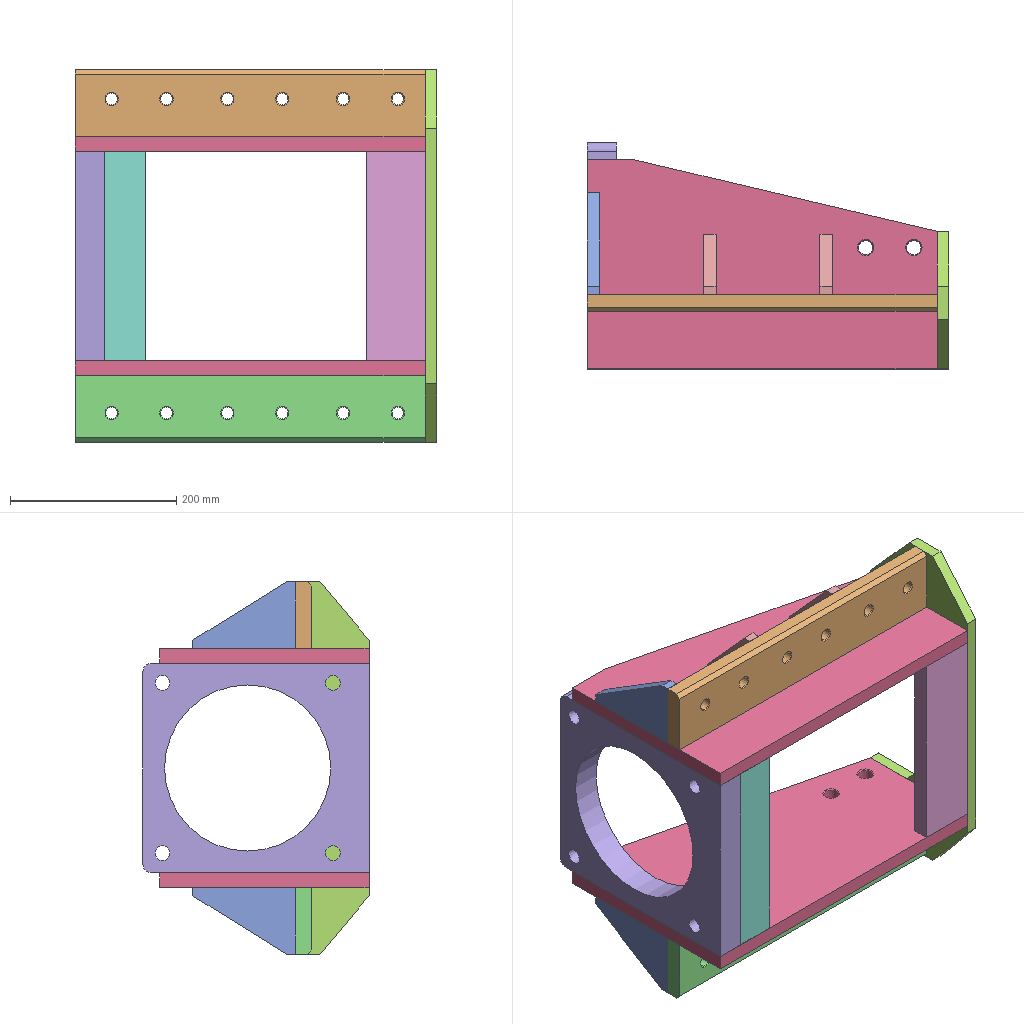Assembly | NX | 9 different items | 14 placed | box 435 x 272 x 448 mm
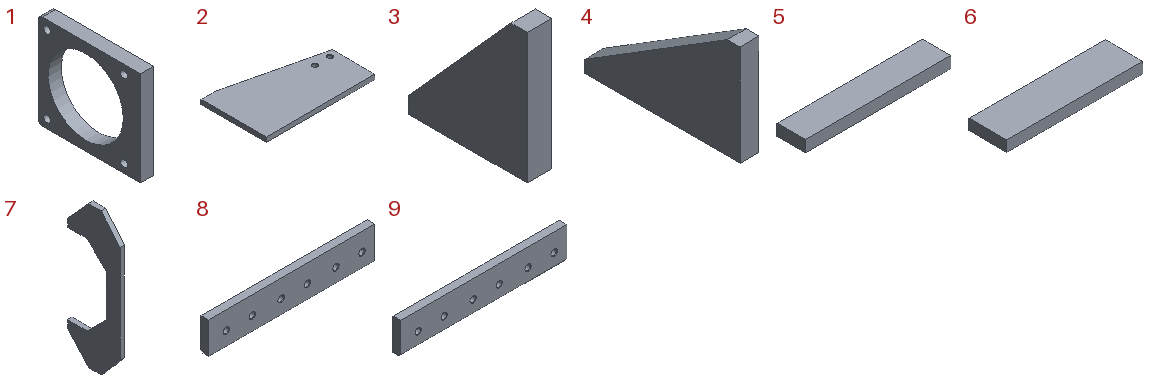Parts list (item | quantity | size | volume | features):
1 | x1 | 35 x 272 x 252 mm | 1262355 mm3 | features BREP 1, DATUM_CSYS 1
2 | x2 | 421 x 252 x 18 mm | 1615279 mm3 | features BREP 1
3 | x4 | 15 x 73 x 80 mm | 54525 mm3 | features BREP 1, DATUM_CSYS 1
4 | x2 | 15 x 123 x 80 mm | 88275 mm3 | features BREP 1, DATUM_CSYS 1
5 | x1 | 252 x 49 x 20 mm | 246960 mm3 | features DATUM_CSYS 2, EXTRUDE 1, SKETCH 1
6 | x1 | 252 x 70 x 20 mm | 352800 mm3 | features DATUM_CSYS 2, EXTRUDE 1, SKETCH 1
7 | x1 | 14 x 165.316 x 448 mm | 531264 mm3 | features REPLACE_FACE 4, DATUM_CSYS 3, EXTRUDE 2, LINKED_FACE 2, SKETCH 2, BREP 1
8 | x1 | 421 x 20 x 80 mm | 649588 mm3 | features SIMPLE HOLE 6, SYMBOLIC_THREAD 6, DATUM_CSYS 3, SKETCH 2, CHAMFER 1, EXTRUDE 1, HOLE PACKAGE 1, LINKED_FACE 1
9 | x1 | 421 x 20 x 80 mm | 649588 mm3 | features SIMPLE HOLE 6, SYMBOLIC_THREAD 6, DATUM_CSYS 3, SKETCH 2, CHAMFER 1, EXTRUDE 1, HOLE PACKAGE 1, LINKED_FACE 1
Mates (type | each side: item.copy, entity, surface, feature):
Fix | assembly component | 2 times
Bond | 2.1 component | assembly component | 2 times
LinearPattern | assembly axis | assembly csys | assembly csys | 3 times
Fix | 1.1 component
Touch | 2.1 face plane Body(5) | 1.1 face plane Body(4) | 3 times
Touch | 9.1 face plane Extrude(1) | 2.1 face plane Body(5) | 2 times
Distance | 9.1 face plane Extrude(1) | 2.1 face plane Body(5)
Touch | 8.1 face plane Extrude(1) | 1.1 face plane Body(4)
Touch | 8.1 face plane Extrude(1) | 2.1 face plane Body(5)
Distance | 8.1 face plane Extrude(1) | 2.1 face plane Body(5)
Touch | 5.1 face plane Extrude(2) | 1.1 face plane Body(4) | 2 times
Touch | 5.1 face plane Extrude(2) | 2.1 face plane Body(5)
Touch | 6.1 face plane Extrude(2) | 2.1 face plane Body(5) | 3 times
Touch | 7.1 face plane Body(1) | 2.1 face plane Body(5) | 2 times
Touch | 7.1 face plane Body(1) | 9.1 face plane Extrude(1)
Touch | 3.1 face plane Body(1) | 8.1 face plane Extrude(1)
Touch | 4.1 face plane Body(1) | 8.1 face plane Extrude(1)
Touch | 3.1 face plane Body(1) | 2.1 face plane Body(5) | 2 times
Touch | 4.1 face plane Body(1) | 2.1 face plane Body(5) | 3 times
Distance | 3.1 face plane Body(1) | 7.1 face plane Body(1) | 2 times
Touch | 3.1 face plane Body(1) | 9.1 face plane Extrude(1)
Touch | 4.1 face plane Body(1) | 1.1 face plane Body(4)
Touch | 4.1 edge | 9.1 face plane Extrude(1)
Bond | 3.1 component | assembly component | 4 times